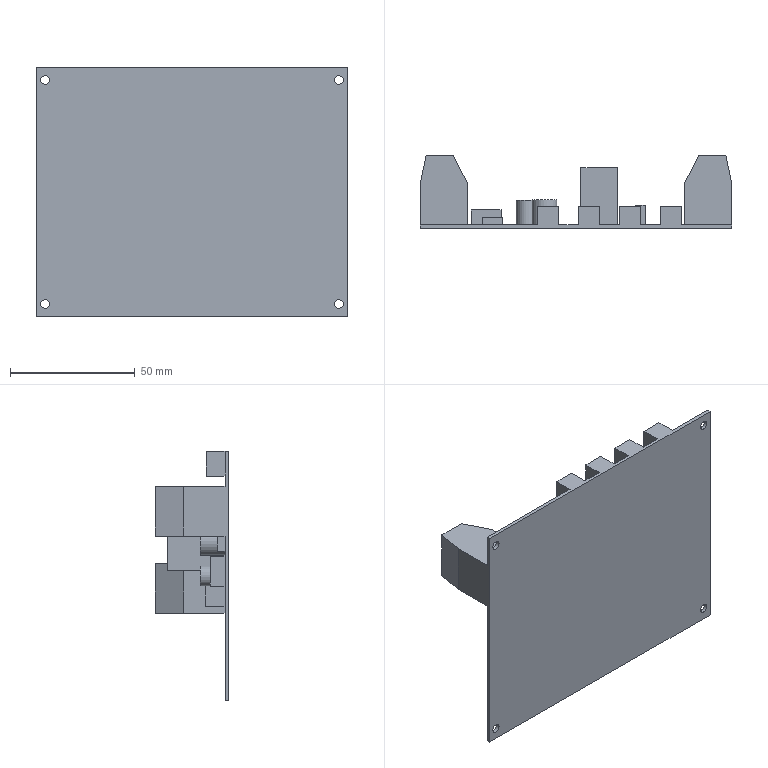Part | NX | features BREP 1 | 1 solid | 62 faces | box 125 x 29.5 x 100 mm | volume 49439 mm3 | plane 56 | cylinder 6 | commonest cylinder face diameters 3.5 x4 8 x1 10 x1